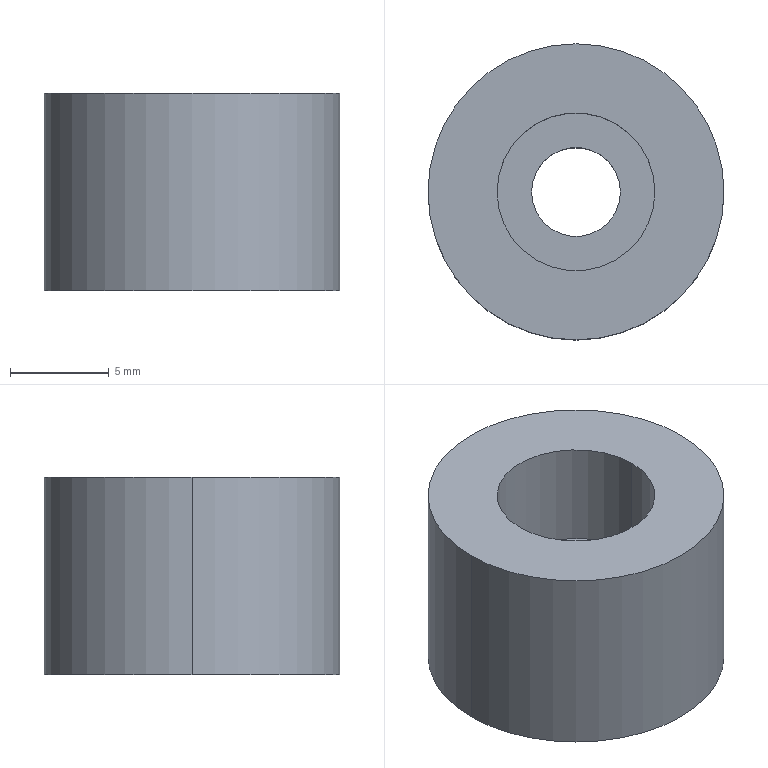Part | NX | features BREP 1 | 1 solid | 9 faces | box 15 x 15 x 10 mm | volume 1419 mm3 | cylinder 6 | plane 3 | commonest cylinder face diameters 4.5 x2 8 x2 15 x2
STEP:
#1=CARTESIAN_POINT('',(-4.,0.,10.));
#2=VERTEX_POINT('',#1);
#3=CARTESIAN_POINT('',(-4.,0.,4.5));
#4=VERTEX_POINT('',#3);
#5=CARTESIAN_POINT('',(-4.,0.,10.));
#6=DIRECTION('',(0.,0.,1.));
#7=VECTOR('',#6,1000.);
#8=LINE('',#5,#7);
#9=EDGE_CURVE('',#2,#4,#8,.F.);
#10=ORIENTED_EDGE('',*,*,#9,.T.);
#11=CARTESIAN_POINT('',(4.,0.,4.5));
#12=VERTEX_POINT('',#11);
#13=CARTESIAN_POINT('',(0.,0.,4.5));
#14=DIRECTION('',(0.,0.,1.));
#15=DIRECTION('',(1.,0.,0.));
#16=AXIS2_PLACEMENT_3D('',#13,#14,#15);
#17=CIRCLE('',#16,4.);
#18=EDGE_CURVE('',#12,#4,#17,.T.);
#19=ORIENTED_EDGE('',*,*,#18,.F.);
#20=CARTESIAN_POINT('',(4.,0.,10.));
#21=VERTEX_POINT('',#20);
#22=CARTESIAN_POINT('',(4.,0.,10.));
#23=DIRECTION('',(0.,0.,1.));
#24=VECTOR('',#23,1000.);
#25=LINE('',#22,#24);
#26=EDGE_CURVE('',#21,#12,#25,.F.);
#27=ORIENTED_EDGE('',*,*,#26,.F.);
#28=CARTESIAN_POINT('',(0.,0.,10.));
#29=DIRECTION('',(0.,0.,1.));
#30=DIRECTION('',(1.,0.,0.));
#31=AXIS2_PLACEMENT_3D('',#28,#29,#30);
#32=CIRCLE('',#31,4.);
#33=EDGE_CURVE('',#21,#2,#32,.T.);
#34=ORIENTED_EDGE('',*,*,#33,.T.);
#35=EDGE_LOOP('',(#10,#19,#27,#34));
#36=FACE_BOUND('',#35,.T.);
#37=CARTESIAN_POINT('',(0.,0.,10.));
#38=DIRECTION('',(0.,0.,1.));
#39=DIRECTION('',(1.,0.,0.));
#40=AXIS2_PLACEMENT_3D('',#37,#38,#39);
#41=CYLINDRICAL_SURFACE('',#40,4.);
#42=ADVANCED_FACE('',(#36),#41,.F.);
#43=ORIENTED_EDGE('',*,*,#18,.T.);
#44=CARTESIAN_POINT('',(0.,0.,4.5));
#45=DIRECTION('',(0.,0.,1.));
#46=DIRECTION('',(1.,0.,0.));
#47=AXIS2_PLACEMENT_3D('',#44,#45,#46);
#48=CIRCLE('',#47,4.);
#49=EDGE_CURVE('',#4,#12,#48,.T.);
#50=ORIENTED_EDGE('',*,*,#49,.T.);
#51=EDGE_LOOP('',(#43,#50));
#52=FACE_BOUND('',#51,.T.);
#53=CARTESIAN_POINT('',(2.25,0.,4.5));
#54=VERTEX_POINT('',#53);
#55=CARTESIAN_POINT('',(-2.25,0.,4.5));
#56=VERTEX_POINT('',#55);
#57=CARTESIAN_POINT('',(0.,0.,4.5));
#58=DIRECTION('',(0.,0.,1.));
#59=DIRECTION('',(1.,0.,0.));
#60=AXIS2_PLACEMENT_3D('',#57,#58,#59);
#61=CIRCLE('',#60,2.25);
#62=EDGE_CURVE('',#54,#56,#61,.T.);
#63=ORIENTED_EDGE('',*,*,#62,.F.);
#64=CARTESIAN_POINT('',(0.,0.,4.5));
#65=DIRECTION('',(0.,0.,1.));
#66=DIRECTION('',(1.,0.,0.));
#67=AXIS2_PLACEMENT_3D('',#64,#65,#66);
#68=CIRCLE('',#67,2.25);
#69=EDGE_CURVE('',#56,#54,#68,.T.);
#70=ORIENTED_EDGE('',*,*,#69,.F.);
#71=EDGE_LOOP('',(#63,#70));
#72=FACE_BOUND('',#71,.T.);
#73=CARTESIAN_POINT('',(2.25,0.,4.5));
#74=DIRECTION('',(0.,0.,-1.));
#75=DIRECTION('',(-1.,0.,0.));
#76=AXIS2_PLACEMENT_3D('',#73,#74,#75);
#77=PLANE('',#76);
#78=ADVANCED_FACE('',(#52,#72),#77,.F.);
#79=CARTESIAN_POINT('',(-2.25,0.,0.));
#80=VERTEX_POINT('',#79);
#81=CARTESIAN_POINT('',(-2.25,0.,10.));
#82=DIRECTION('',(0.,0.,1.));
#83=VECTOR('',#82,1000.);
#84=LINE('',#81,#83);
#85=EDGE_CURVE('',#56,#80,#84,.F.);
#86=ORIENTED_EDGE('',*,*,#85,.T.);
#87=CARTESIAN_POINT('',(2.25,0.,0.));
#88=VERTEX_POINT('',#87);
#89=CARTESIAN_POINT('',(0.,0.,0.));
#90=DIRECTION('',(0.,0.,1.));
#91=DIRECTION('',(1.,0.,0.));
#92=AXIS2_PLACEMENT_3D('',#89,#90,#91);
#93=CIRCLE('',#92,2.25);
#94=EDGE_CURVE('',#88,#80,#93,.T.);
#95=ORIENTED_EDGE('',*,*,#94,.F.);
#96=CARTESIAN_POINT('',(2.25,0.,10.));
#97=DIRECTION('',(0.,0.,1.));
#98=VECTOR('',#97,1000.);
#99=LINE('',#96,#98);
#100=EDGE_CURVE('',#54,#88,#99,.F.);
#101=ORIENTED_EDGE('',*,*,#100,.F.);
#102=ORIENTED_EDGE('',*,*,#62,.T.);
#103=EDGE_LOOP('',(#86,#95,#101,#102));
#104=FACE_BOUND('',#103,.T.);
#105=CARTESIAN_POINT('',(0.,0.,10.));
#106=DIRECTION('',(0.,0.,1.));
#107=DIRECTION('',(1.,0.,0.));
#108=AXIS2_PLACEMENT_3D('',#105,#106,#107);
#109=CYLINDRICAL_SURFACE('',#108,2.25);
#110=ADVANCED_FACE('',(#104),#109,.F.);
#111=CARTESIAN_POINT('',(-7.5,0.,0.));
#112=VERTEX_POINT('',#111);
#113=CARTESIAN_POINT('',(7.5,0.,0.));
#114=VERTEX_POINT('',#113);
#115=CARTESIAN_POINT('',(0.,0.,0.));
#116=DIRECTION('',(0.,0.,1.));
#117=DIRECTION('',(1.,0.,0.));
#118=AXIS2_PLACEMENT_3D('',#115,#116,#117);
#119=CIRCLE('',#118,7.5);
#120=EDGE_CURVE('',#112,#114,#119,.T.);
#121=ORIENTED_EDGE('',*,*,#120,.F.);
#122=CARTESIAN_POINT('',(0.,0.,0.));
#123=DIRECTION('',(0.,0.,1.));
#124=DIRECTION('',(1.,0.,0.));
#125=AXIS2_PLACEMENT_3D('',#122,#123,#124);
#126=CIRCLE('',#125,7.5);
#127=EDGE_CURVE('',#114,#112,#126,.T.);
#128=ORIENTED_EDGE('',*,*,#127,.F.);
#129=EDGE_LOOP('',(#121,#128));
#130=FACE_BOUND('',#129,.T.);
#131=ORIENTED_EDGE('',*,*,#94,.T.);
#132=CARTESIAN_POINT('',(0.,0.,0.));
#133=DIRECTION('',(0.,0.,1.));
#134=DIRECTION('',(1.,0.,0.));
#135=AXIS2_PLACEMENT_3D('',#132,#133,#134);
#136=CIRCLE('',#135,2.25);
#137=EDGE_CURVE('',#80,#88,#136,.T.);
#138=ORIENTED_EDGE('',*,*,#137,.T.);
#139=EDGE_LOOP('',(#131,#138));
#140=FACE_BOUND('',#139,.T.);
#141=CARTESIAN_POINT('',(0.,0.,0.));
#142=DIRECTION('',(0.,0.,1.));
#143=DIRECTION('',(1.,0.,0.));
#144=AXIS2_PLACEMENT_3D('',#141,#142,#143);
#145=PLANE('',#144);
#146=ADVANCED_FACE('',(#130,#140),#145,.F.);
#147=CARTESIAN_POINT('',(-7.5,0.,10.));
#148=VERTEX_POINT('',#147);
#149=CARTESIAN_POINT('',(7.5,0.,10.));
#150=VERTEX_POINT('',#149);
#151=CARTESIAN_POINT('',(0.,0.,10.));
#152=DIRECTION('',(0.,0.,1.));
#153=DIRECTION('',(1.,0.,0.));
#154=AXIS2_PLACEMENT_3D('',#151,#152,#153);
#155=CIRCLE('',#154,7.5);
#156=EDGE_CURVE('',#148,#150,#155,.T.);
#157=ORIENTED_EDGE('',*,*,#156,.T.);
#158=CARTESIAN_POINT('',(0.,0.,10.));
#159=DIRECTION('',(0.,0.,1.));
#160=DIRECTION('',(1.,0.,0.));
#161=AXIS2_PLACEMENT_3D('',#158,#159,#160);
#162=CIRCLE('',#161,7.5);
#163=EDGE_CURVE('',#150,#148,#162,.T.);
#164=ORIENTED_EDGE('',*,*,#163,.T.);
#165=EDGE_LOOP('',(#157,#164));
#166=FACE_BOUND('',#165,.T.);
#167=ORIENTED_EDGE('',*,*,#33,.F.);
#168=CARTESIAN_POINT('',(0.,0.,10.));
#169=DIRECTION('',(0.,0.,1.));
#170=DIRECTION('',(1.,0.,0.));
#171=AXIS2_PLACEMENT_3D('',#168,#169,#170);
#172=CIRCLE('',#171,4.);
#173=EDGE_CURVE('',#2,#21,#172,.T.);
#174=ORIENTED_EDGE('',*,*,#173,.F.);
#175=EDGE_LOOP('',(#167,#174));
#176=FACE_BOUND('',#175,.T.);
#177=CARTESIAN_POINT('',(0.,0.,10.));
#178=DIRECTION('',(0.,0.,1.));
#179=DIRECTION('',(1.,0.,0.));
#180=AXIS2_PLACEMENT_3D('',#177,#178,#179);
#181=PLANE('',#180);
#182=ADVANCED_FACE('',(#166,#176),#181,.T.);
#183=CARTESIAN_POINT('',(7.5,0.,10.));
#184=DIRECTION('',(0.,0.,-1.));
#185=VECTOR('',#184,1000.);
#186=LINE('',#183,#185);
#187=EDGE_CURVE('',#150,#114,#186,.T.);
#188=ORIENTED_EDGE('',*,*,#187,.F.);
#189=ORIENTED_EDGE('',*,*,#156,.F.);
#190=CARTESIAN_POINT('',(-7.5,0.,10.));
#191=DIRECTION('',(0.,0.,-1.));
#192=VECTOR('',#191,1000.);
#193=LINE('',#190,#192);
#194=EDGE_CURVE('',#148,#112,#193,.T.);
#195=ORIENTED_EDGE('',*,*,#194,.T.);
#196=ORIENTED_EDGE('',*,*,#120,.T.);
#197=EDGE_LOOP('',(#188,#189,#195,#196));
#198=FACE_BOUND('',#197,.T.);
#199=CARTESIAN_POINT('',(0.,0.,10.));
#200=DIRECTION('',(0.,0.,-1.));
#201=DIRECTION('',(-1.,0.,0.));
#202=AXIS2_PLACEMENT_3D('',#199,#200,#201);
#203=CYLINDRICAL_SURFACE('',#202,7.5);
#204=ADVANCED_FACE('',(#198),#203,.T.);
#205=ORIENTED_EDGE('',*,*,#163,.F.);
#206=ORIENTED_EDGE('',*,*,#187,.T.);
#207=ORIENTED_EDGE('',*,*,#127,.T.);
#208=ORIENTED_EDGE('',*,*,#194,.F.);
#209=EDGE_LOOP('',(#205,#206,#207,#208));
#210=FACE_BOUND('',#209,.T.);
#211=CARTESIAN_POINT('',(0.,0.,10.));
#212=DIRECTION('',(0.,0.,-1.));
#213=DIRECTION('',(-1.,0.,0.));
#214=AXIS2_PLACEMENT_3D('',#211,#212,#213);
#215=CYLINDRICAL_SURFACE('',#214,7.5);
#216=ADVANCED_FACE('',(#210),#215,.T.);
#217=ORIENTED_EDGE('',*,*,#137,.F.);
#218=ORIENTED_EDGE('',*,*,#85,.F.);
#219=ORIENTED_EDGE('',*,*,#69,.T.);
#220=ORIENTED_EDGE('',*,*,#100,.T.);
#221=EDGE_LOOP('',(#217,#218,#219,#220));
#222=FACE_BOUND('',#221,.T.);
#223=CARTESIAN_POINT('',(0.,0.,10.));
#224=DIRECTION('',(0.,0.,1.));
#225=DIRECTION('',(1.,0.,0.));
#226=AXIS2_PLACEMENT_3D('',#223,#224,#225);
#227=CYLINDRICAL_SURFACE('',#226,2.25);
#228=ADVANCED_FACE('',(#222),#227,.F.);
#229=ORIENTED_EDGE('',*,*,#49,.F.);
#230=ORIENTED_EDGE('',*,*,#9,.F.);
#231=ORIENTED_EDGE('',*,*,#173,.T.);
#232=ORIENTED_EDGE('',*,*,#26,.T.);
#233=EDGE_LOOP('',(#229,#230,#231,#232));
#234=FACE_BOUND('',#233,.T.);
#235=CARTESIAN_POINT('',(0.,0.,10.));
#236=DIRECTION('',(0.,0.,1.));
#237=DIRECTION('',(1.,0.,0.));
#238=AXIS2_PLACEMENT_3D('',#235,#236,#237);
#239=CYLINDRICAL_SURFACE('',#238,4.);
#240=ADVANCED_FACE('',(#234),#239,.F.);
#241=CLOSED_SHELL('',(#42,#78,#110,#146,#182,#204,#216,#228,#240));
#242=MANIFOLD_SOLID_BREP('',#241);
#243=(LENGTH_UNIT()NAMED_UNIT(*)SI_UNIT(.MILLI.,.METRE.));
#244=UNCERTAINTY_MEASURE_WITH_UNIT(LENGTH_MEASURE(0.00001),#243,'','');
#245=(NAMED_UNIT(*)PLANE_ANGLE_UNIT()SI_UNIT($,.RADIAN.));
#246=(NAMED_UNIT(*)SI_UNIT($,.STERADIAN.)SOLID_ANGLE_UNIT());
#247=(GEOMETRIC_REPRESENTATION_CONTEXT(3)GLOBAL_UNCERTAINTY_ASSIGNED_CONTEXT((#244))GLOBAL_UNIT_ASSIGNED_CONTEXT((#243,#245,#246))REPRESENTATION_CONTEXT('',''));
#248=ADVANCED_BREP_SHAPE_REPRESENTATION('',(#242),#247);